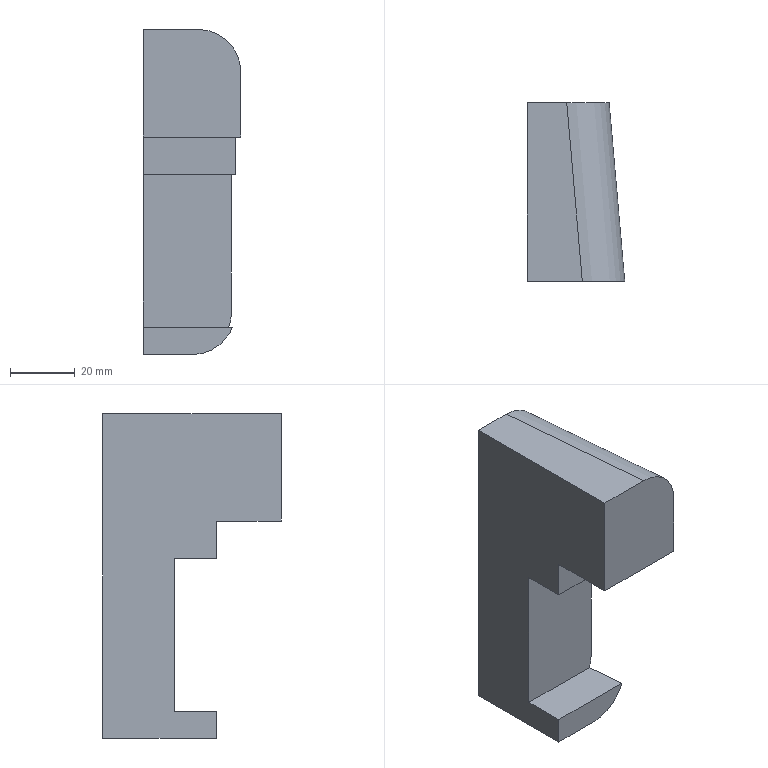Part | STEP file | 1 solid | 14 faces | box 30 x 55 x 100 mm | volume 92612 mm3 | plane 12 | cylinder 2 | commonest cylinder face diameters 26 x2
STEP:
#1=CARTESIAN_POINT('',(0.,0.,0.));
#2=DIRECTION('',(0.,0.,1.));
#3=DIRECTION('',(1.,0.,0.));
#4=AXIS2_PLACEMENT_3D('',#1,#2,#3);
#5=CARTESIAN_POINT('',(37.138,70.5,195.451));
#6=VERTEX_POINT('',#5);
#7=CARTESIAN_POINT('',(37.138,90.5,195.451));
#8=VERTEX_POINT('',#7);
#9=CARTESIAN_POINT('',(37.138,90.366,195.451));
#10=DIRECTION('',(0.,1.,0.));
#11=VECTOR('',#10,1.);
#12=LINE('',#9,#11);
#13=CARTESIAN_POINT('',(37.138,-9.5,128.53));
#14=DIRECTION('',(1.,0.,0.));
#15=DIRECTION('',(0.,0.,-1.));
#16=AXIS2_PLACEMENT_3D('',#13,#14,#15);
#17=PLANE('',#16);
#18=CARTESIAN_POINT('',(-66.922,99.866));
#19=DIRECTION('',(0.,1.));
#20=VECTOR('',#19,1.);
#21=LINE('',#18,#20);
#22=(GEOMETRIC_REPRESENTATION_CONTEXT(2)PARAMETRIC_REPRESENTATION_CONTEXT()REPRESENTATION_CONTEXT('',''));
#23=DEFINITIONAL_REPRESENTATION('',(#21),#22);
#24=PCURVE('',#17,#23);
#25=CARTESIAN_POINT('',(47.086,69.939,195.451));
#26=DIRECTION('',(0.,0.,-1.));
#27=DIRECTION('',(-1.,0.,0.));
#28=AXIS2_PLACEMENT_3D('',#25,#26,#27);
#29=PLANE('',#28);
#30=CARTESIAN_POINT('',(9.948,20.427));
#31=DIRECTION('',(0.,1.));
#32=VECTOR('',#31,1.);
#33=LINE('',#30,#32);
#34=(GEOMETRIC_REPRESENTATION_CONTEXT(2)PARAMETRIC_REPRESENTATION_CONTEXT()REPRESENTATION_CONTEXT('',''));
#35=DEFINITIONAL_REPRESENTATION('',(#33),#34);
#36=PCURVE('',#29,#35);
#37=SURFACE_CURVE('',#12,(#24,#36),.PCURVE_S1.);
#38=EDGE_CURVE('',#6,#8,#37,.T.);
#39=ORIENTED_EDGE('',*,*,#38,.F.);
#40=CARTESIAN_POINT('',(37.138,70.5,228.53));
#41=VERTEX_POINT('',#40);
#42=CARTESIAN_POINT('',(37.138,70.5,128.53));
#43=DIRECTION('',(0.,0.,1.));
#44=VECTOR('',#43,1.);
#45=LINE('',#42,#44);
#46=CARTESIAN_POINT('',(0.,80.));
#47=DIRECTION('',(-1.,0.));
#48=VECTOR('',#47,1.);
#49=LINE('',#46,#48);
#50=(GEOMETRIC_REPRESENTATION_CONTEXT(2)PARAMETRIC_REPRESENTATION_CONTEXT()REPRESENTATION_CONTEXT('',''));
#51=DEFINITIONAL_REPRESENTATION('',(#49),#50);
#52=PCURVE('',#17,#51);
#53=CARTESIAN_POINT('',(-72.862,70.5,-363.47));
#54=DIRECTION('',(0.,1.,0.));
#55=DIRECTION('',(0.,0.,-1.));
#56=AXIS2_PLACEMENT_3D('',#53,#54,#55);
#57=PLANE('',#56);
#58=CARTESIAN_POINT('',(-492.,-110.));
#59=DIRECTION('',(-1.,0.));
#60=VECTOR('',#59,1.);
#61=LINE('',#58,#60);
#62=(GEOMETRIC_REPRESENTATION_CONTEXT(2)PARAMETRIC_REPRESENTATION_CONTEXT()REPRESENTATION_CONTEXT('',''));
#63=DEFINITIONAL_REPRESENTATION('',(#61),#62);
#64=PCURVE('',#57,#63);
#65=SURFACE_CURVE('',#45,(#52,#64),.PCURVE_S1.);
#66=EDGE_CURVE('',#6,#41,#65,.T.);
#67=ORIENTED_EDGE('',*,*,#66,.T.);
#68=CARTESIAN_POINT('',(37.138,125.5,228.53));
#69=VERTEX_POINT('',#68);
#70=CARTESIAN_POINT('',(37.138,-9.5,228.53));
#71=DIRECTION('',(0.,1.,0.));
#72=VECTOR('',#71,1.);
#73=LINE('',#70,#72);
#74=CARTESIAN_POINT('',(-100.,0.));
#75=DIRECTION('',(0.,1.));
#76=VECTOR('',#75,1.);
#77=LINE('',#74,#76);
#78=(GEOMETRIC_REPRESENTATION_CONTEXT(2)PARAMETRIC_REPRESENTATION_CONTEXT()REPRESENTATION_CONTEXT('',''));
#79=DEFINITIONAL_REPRESENTATION('',(#77),#78);
#80=PCURVE('',#17,#79);
#81=CARTESIAN_POINT('',(37.138,-9.5,228.53));
#82=DIRECTION('',(0.,0.,-1.));
#83=DIRECTION('',(-1.,0.,0.));
#84=AXIS2_PLACEMENT_3D('',#81,#82,#83);
#85=PLANE('',#84);
#86=CARTESIAN_POINT('',(0.,0.));
#87=DIRECTION('',(0.,1.));
#88=VECTOR('',#87,1.);
#89=LINE('',#86,#88);
#90=(GEOMETRIC_REPRESENTATION_CONTEXT(2)PARAMETRIC_REPRESENTATION_CONTEXT()REPRESENTATION_CONTEXT('',''));
#91=DEFINITIONAL_REPRESENTATION('',(#89),#90);
#92=PCURVE('',#85,#91);
#93=SURFACE_CURVE('',#73,(#80,#92),.PCURVE_S1.);
#94=EDGE_CURVE('',#41,#69,#93,.T.);
#95=ORIENTED_EDGE('',*,*,#94,.T.);
#96=CARTESIAN_POINT('',(37.138,125.5,128.53));
#97=VERTEX_POINT('',#96);
#98=CARTESIAN_POINT('',(37.138,125.5,128.53));
#99=DIRECTION('',(0.,0.,-1.));
#100=VECTOR('',#99,1.);
#101=LINE('',#98,#100);
#102=CARTESIAN_POINT('',(0.,135.));
#103=DIRECTION('',(1.,0.));
#104=VECTOR('',#103,1.);
#105=LINE('',#102,#104);
#106=(GEOMETRIC_REPRESENTATION_CONTEXT(2)PARAMETRIC_REPRESENTATION_CONTEXT()REPRESENTATION_CONTEXT('',''));
#107=DEFINITIONAL_REPRESENTATION('',(#105),#106);
#108=PCURVE('',#17,#107);
#109=CARTESIAN_POINT('',(-72.362,125.5,-51.47));
#110=DIRECTION('',(0.,-1.,0.));
#111=DIRECTION('',(0.,0.,-1.));
#112=AXIS2_PLACEMENT_3D('',#109,#110,#111);
#113=PLANE('',#112);
#114=CARTESIAN_POINT('',(-180.,109.5));
#115=DIRECTION('',(1.,0.));
#116=VECTOR('',#115,1.);
#117=LINE('',#114,#116);
#118=(GEOMETRIC_REPRESENTATION_CONTEXT(2)PARAMETRIC_REPRESENTATION_CONTEXT()REPRESENTATION_CONTEXT('',''));
#119=DEFINITIONAL_REPRESENTATION('',(#117),#118);
#120=PCURVE('',#113,#119);
#121=SURFACE_CURVE('',#101,(#108,#120),.PCURVE_S1.);
#122=EDGE_CURVE('',#69,#97,#121,.T.);
#123=ORIENTED_EDGE('',*,*,#122,.T.);
#124=CARTESIAN_POINT('',(37.138,90.5,128.53));
#125=VERTEX_POINT('',#124);
#126=CARTESIAN_POINT('',(37.138,-9.5,128.53));
#127=DIRECTION('',(0.,1.,0.));
#128=VECTOR('',#127,1.);
#129=LINE('',#126,#128);
#130=CARTESIAN_POINT('',(0.,0.));
#131=DIRECTION('',(0.,1.));
#132=VECTOR('',#131,1.);
#133=LINE('',#130,#132);
#134=(GEOMETRIC_REPRESENTATION_CONTEXT(2)PARAMETRIC_REPRESENTATION_CONTEXT()REPRESENTATION_CONTEXT('',''));
#135=DEFINITIONAL_REPRESENTATION('',(#133),#134);
#136=PCURVE('',#17,#135);
#137=CARTESIAN_POINT('',(57.138,-9.5,128.53));
#138=DIRECTION('',(0.,0.,1.));
#139=DIRECTION('',(1.,0.,0.));
#140=AXIS2_PLACEMENT_3D('',#137,#138,#139);
#141=PLANE('',#140);
#142=CARTESIAN_POINT('',(-20.,0.));
#143=DIRECTION('',(0.,1.));
#144=VECTOR('',#143,1.);
#145=LINE('',#142,#144);
#146=(GEOMETRIC_REPRESENTATION_CONTEXT(2)PARAMETRIC_REPRESENTATION_CONTEXT()REPRESENTATION_CONTEXT('',''));
#147=DEFINITIONAL_REPRESENTATION('',(#145),#146);
#148=PCURVE('',#141,#147);
#149=SURFACE_CURVE('',#129,(#136,#148),.PCURVE_S1.);
#150=EDGE_CURVE('',#125,#97,#149,.T.);
#151=ORIENTED_EDGE('',*,*,#150,.F.);
#152=CARTESIAN_POINT('',(37.138,90.5,136.951));
#153=VERTEX_POINT('',#152);
#154=CARTESIAN_POINT('',(37.138,90.5,128.53));
#155=DIRECTION('',(0.,0.,1.));
#156=VECTOR('',#155,1.);
#157=LINE('',#154,#156);
#158=CARTESIAN_POINT('',(0.,100.));
#159=DIRECTION('',(-1.,0.));
#160=VECTOR('',#159,1.);
#161=LINE('',#158,#160);
#162=(GEOMETRIC_REPRESENTATION_CONTEXT(2)PARAMETRIC_REPRESENTATION_CONTEXT()REPRESENTATION_CONTEXT('',''));
#163=DEFINITIONAL_REPRESENTATION('',(#161),#162);
#164=PCURVE('',#17,#163);
#165=CARTESIAN_POINT('',(47.086,90.5,125.451));
#166=DIRECTION('',(0.,1.,0.));
#167=DIRECTION('',(0.,0.,1.));
#168=AXIS2_PLACEMENT_3D('',#165,#166,#167);
#169=PLANE('',#168);
#170=CARTESIAN_POINT('',(3.078,-9.948));
#171=DIRECTION('',(1.,0.));
#172=VECTOR('',#171,1.);
#173=LINE('',#170,#172);
#174=(GEOMETRIC_REPRESENTATION_CONTEXT(2)PARAMETRIC_REPRESENTATION_CONTEXT()REPRESENTATION_CONTEXT('',''));
#175=DEFINITIONAL_REPRESENTATION('',(#173),#174);
#176=PCURVE('',#169,#175);
#177=SURFACE_CURVE('',#157,(#164,#176),.PCURVE_S1.);
#178=EDGE_CURVE('',#125,#153,#177,.T.);
#179=ORIENTED_EDGE('',*,*,#178,.T.);
#180=CARTESIAN_POINT('',(37.138,103.5,136.951));
#181=VERTEX_POINT('',#180);
#182=CARTESIAN_POINT('',(37.138,69.939,136.951));
#183=DIRECTION('',(0.,1.,0.));
#184=VECTOR('',#183,1.);
#185=LINE('',#182,#184);
#186=CARTESIAN_POINT('',(-8.422,79.439));
#187=DIRECTION('',(0.,1.));
#188=VECTOR('',#187,1.);
#189=LINE('',#186,#188);
#190=(GEOMETRIC_REPRESENTATION_CONTEXT(2)PARAMETRIC_REPRESENTATION_CONTEXT()REPRESENTATION_CONTEXT('',''));
#191=DEFINITIONAL_REPRESENTATION('',(#189),#190);
#192=PCURVE('',#17,#191);
#193=CARTESIAN_POINT('',(47.085,69.939,136.951));
#194=DIRECTION('',(0.,0.,1.));
#195=DIRECTION('',(-1.,0.,0.));
#196=AXIS2_PLACEMENT_3D('',#193,#194,#195);
#197=PLANE('',#196);
#198=CARTESIAN_POINT('',(9.948,0.));
#199=DIRECTION('',(0.,-1.));
#200=VECTOR('',#199,1.);
#201=LINE('',#198,#200);
#202=(GEOMETRIC_REPRESENTATION_CONTEXT(2)PARAMETRIC_REPRESENTATION_CONTEXT()REPRESENTATION_CONTEXT('',''));
#203=DEFINITIONAL_REPRESENTATION('',(#201),#202);
#204=PCURVE('',#197,#203);
#205=SURFACE_CURVE('',#185,(#192,#204),.PCURVE_S1.);
#206=EDGE_CURVE('',#153,#181,#205,.T.);
#207=ORIENTED_EDGE('',*,*,#206,.T.);
#208=CARTESIAN_POINT('',(37.138,103.5,183.951));
#209=VERTEX_POINT('',#208);
#210=CARTESIAN_POINT('',(37.138,103.5,128.53));
#211=DIRECTION('',(0.,0.,-1.));
#212=VECTOR('',#211,1.);
#213=LINE('',#210,#212);
#214=CARTESIAN_POINT('',(0.,113.));
#215=DIRECTION('',(1.,0.));
#216=VECTOR('',#215,1.);
#217=LINE('',#214,#216);
#218=(GEOMETRIC_REPRESENTATION_CONTEXT(2)PARAMETRIC_REPRESENTATION_CONTEXT()REPRESENTATION_CONTEXT('',''));
#219=DEFINITIONAL_REPRESENTATION('',(#217),#218);
#220=PCURVE('',#17,#219);
#221=CARTESIAN_POINT('',(87.138,103.5,108.53));
#222=DIRECTION('',(0.,-1.,0.));
#223=DIRECTION('',(0.,0.,-1.));
#224=AXIS2_PLACEMENT_3D('',#221,#222,#223);
#225=PLANE('',#224);
#226=CARTESIAN_POINT('',(-20.,-50.));
#227=DIRECTION('',(1.,0.));
#228=VECTOR('',#227,1.);
#229=LINE('',#226,#228);
#230=(GEOMETRIC_REPRESENTATION_CONTEXT(2)PARAMETRIC_REPRESENTATION_CONTEXT()REPRESENTATION_CONTEXT('',''));
#231=DEFINITIONAL_REPRESENTATION('',(#229),#230);
#232=PCURVE('',#225,#231);
#233=SURFACE_CURVE('',#213,(#220,#232),.PCURVE_S1.);
#234=EDGE_CURVE('',#209,#181,#233,.T.);
#235=ORIENTED_EDGE('',*,*,#234,.F.);
#236=CARTESIAN_POINT('',(37.138,90.5,183.951));
#237=VERTEX_POINT('',#236);
#238=CARTESIAN_POINT('',(37.138,69.939,183.951));
#239=DIRECTION('',(0.,1.,0.));
#240=VECTOR('',#239,1.);
#241=LINE('',#238,#240);
#242=CARTESIAN_POINT('',(-55.422,79.439));
#243=DIRECTION('',(0.,1.));
#244=VECTOR('',#243,1.);
#245=LINE('',#242,#244);
#246=(GEOMETRIC_REPRESENTATION_CONTEXT(2)PARAMETRIC_REPRESENTATION_CONTEXT()REPRESENTATION_CONTEXT('',''));
#247=DEFINITIONAL_REPRESENTATION('',(#245),#246);
#248=PCURVE('',#17,#247);
#249=CARTESIAN_POINT('',(47.085,69.939,183.951));
#250=DIRECTION('',(0.,0.,1.));
#251=DIRECTION('',(-1.,0.,0.));
#252=AXIS2_PLACEMENT_3D('',#249,#250,#251);
#253=PLANE('',#252);
#254=CARTESIAN_POINT('',(9.948,0.));
#255=DIRECTION('',(0.,-1.));
#256=VECTOR('',#255,1.);
#257=LINE('',#254,#256);
#258=(GEOMETRIC_REPRESENTATION_CONTEXT(2)PARAMETRIC_REPRESENTATION_CONTEXT()REPRESENTATION_CONTEXT('',''));
#259=DEFINITIONAL_REPRESENTATION('',(#257),#258);
#260=PCURVE('',#253,#259);
#261=SURFACE_CURVE('',#241,(#248,#260),.PCURVE_S1.);
#262=EDGE_CURVE('',#237,#209,#261,.T.);
#263=ORIENTED_EDGE('',*,*,#262,.F.);
#264=CARTESIAN_POINT('',(37.138,90.5,195.451));
#265=DIRECTION('',(0.,0.,-1.));
#266=VECTOR('',#265,1.);
#267=LINE('',#264,#266);
#268=CARTESIAN_POINT('',(-66.922,100.));
#269=DIRECTION('',(1.,0.));
#270=VECTOR('',#269,1.);
#271=LINE('',#268,#270);
#272=(GEOMETRIC_REPRESENTATION_CONTEXT(2)PARAMETRIC_REPRESENTATION_CONTEXT()REPRESENTATION_CONTEXT('',''));
#273=DEFINITIONAL_REPRESENTATION('',(#271),#272);
#274=PCURVE('',#17,#273);
#275=CARTESIAN_POINT('',(47.086,90.5,195.451));
#276=DIRECTION('',(0.,1.,0.));
#277=DIRECTION('',(0.,0.,-1.));
#278=AXIS2_PLACEMENT_3D('',#275,#276,#277);
#279=PLANE('',#278);
#280=CARTESIAN_POINT('',(0.,9.948));
#281=DIRECTION('',(1.,0.));
#282=VECTOR('',#281,1.);
#283=LINE('',#280,#282);
#284=(GEOMETRIC_REPRESENTATION_CONTEXT(2)PARAMETRIC_REPRESENTATION_CONTEXT()REPRESENTATION_CONTEXT('',''));
#285=DEFINITIONAL_REPRESENTATION('',(#283),#284);
#286=PCURVE('',#279,#285);
#287=SURFACE_CURVE('',#267,(#274,#286),.PCURVE_S1.);
#288=EDGE_CURVE('',#8,#237,#287,.T.);
#289=ORIENTED_EDGE('',*,*,#288,.F.);
#290=EDGE_LOOP('',(#39,#67,#95,#123,#151,#179,#207,#235,#263,#289));
#291=FACE_BOUND('',#290,.T.);
#292=ADVANCED_FACE('',(#291),#17,.F.);
#293=CARTESIAN_POINT('',(52.338,90.5,128.53));
#294=VERTEX_POINT('',#293);
#295=CARTESIAN_POINT('',(64.552,90.5,136.951));
#296=VERTEX_POINT('',#295);
#297=CARTESIAN_POINT('',(52.338,90.5,128.53));
#298=CARTESIAN_POINT('',(57.955,90.5,128.53));
#299=CARTESIAN_POINT('',(62.574,90.5,131.714));
#300=CARTESIAN_POINT('',(64.552,90.5,136.951));
#301=(BOUNDED_CURVE()B_SPLINE_CURVE(3,(#297,#298,#299,#300),.UNSPECIFIED.,.F.,.F.)B_SPLINE_CURVE_WITH_KNOTS((4,4),(1.571,2.782),.PIECEWISE_BEZIER_KNOTS.)CURVE()GEOMETRIC_REPRESENTATION_ITEM()RATIONAL_B_SPLINE_CURVE((1.,0.8815,0.8815,1.))REPRESENTATION_ITEM(''));
#302=CARTESIAN_POINT('',(61.057,-9.157,141.53));
#303=DIRECTION('',(-0.08716,0.9962,0.));
#304=DIRECTION('',(0.9962,0.08716,0.));
#305=AXIS2_PLACEMENT_3D('',#302,#303,#304);
#306=CYLINDRICAL_SURFACE('',#305,13.);
#307=CARTESIAN_POINT('',(1.571,100.038));
#308=CARTESIAN_POINT('',(1.554,100.018));
#309=CARTESIAN_POINT('',(1.519,99.979));
#310=CARTESIAN_POINT('',(1.466,99.919));
#311=CARTESIAN_POINT('',(1.412,99.858));
#312=CARTESIAN_POINT('',(1.358,99.797));
#313=CARTESIAN_POINT('',(1.303,99.737));
#314=CARTESIAN_POINT('',(1.247,99.676));
#315=CARTESIAN_POINT('',(1.192,99.617));
#316=CARTESIAN_POINT('',(1.135,99.558));
#317=CARTESIAN_POINT('',(1.079,99.5));
#318=CARTESIAN_POINT('',(1.022,99.444));
#319=CARTESIAN_POINT('',(0.9653,99.39));
#320=CARTESIAN_POINT('',(0.9086,99.338));
#321=CARTESIAN_POINT('',(0.8519,99.288));
#322=CARTESIAN_POINT('',(0.7954,99.241));
#323=CARTESIAN_POINT('',(0.7391,99.197));
#324=CARTESIAN_POINT('',(0.6832,99.155));
#325=CARTESIAN_POINT('',(0.6278,99.117));
#326=CARTESIAN_POINT('',(0.5729,99.082));
#327=CARTESIAN_POINT('',(0.5185,99.049));
#328=CARTESIAN_POINT('',(0.4649,99.021));
#329=CARTESIAN_POINT('',(0.4119,98.995));
#330=CARTESIAN_POINT('',(0.3771,98.98));
#331=CARTESIAN_POINT('',(0.3599,98.973));
#332=B_SPLINE_CURVE_WITH_KNOTS('',3,(#307,#308,#309,#310,#311,#312,#313,#314,#315,#316,#317,#318,#319,#320,#321,#322,#323,#324,#325,#326,#327,#328,#329,#330,#331),.UNSPECIFIED.,.F.,.F.,(4,1,1,1,1,1,1,1,1,1,1,1,1,1,1,1,1,1,1,1,1,1,4),(1.571,1.626,1.681,1.736,1.791,1.846,1.901,1.956,2.011,2.066,2.121,2.176,2.231,2.286,2.341,2.396,2.451,2.506,2.562,2.617,2.672,2.727,2.782),.QUASI_UNIFORM_KNOTS.);
#333=(GEOMETRIC_REPRESENTATION_CONTEXT(2)PARAMETRIC_REPRESENTATION_CONTEXT()REPRESENTATION_CONTEXT('',''));
#334=DEFINITIONAL_REPRESENTATION('',(#332),#333);
#335=PCURVE('',#306,#334);
#336=CARTESIAN_POINT('',(3.078,5.253));
#337=CARTESIAN_POINT('',(3.078,10.87));
#338=CARTESIAN_POINT('',(6.263,15.488));
#339=CARTESIAN_POINT('',(11.5,17.466));
#340=(BOUNDED_CURVE()B_SPLINE_CURVE(3,(#336,#337,#338,#339),.UNSPECIFIED.,.F.,.F.)B_SPLINE_CURVE_WITH_KNOTS((4,4),(1.571,2.782),.PIECEWISE_BEZIER_KNOTS.)CURVE()GEOMETRIC_REPRESENTATION_ITEM()RATIONAL_B_SPLINE_CURVE((1.,0.8815,0.8815,1.))REPRESENTATION_ITEM(''));
#341=(GEOMETRIC_REPRESENTATION_CONTEXT(2)PARAMETRIC_REPRESENTATION_CONTEXT()REPRESENTATION_CONTEXT('',''));
#342=DEFINITIONAL_REPRESENTATION('',(#340),#341);
#343=PCURVE('',#169,#342);
#344=SURFACE_CURVE('',#301,(#335,#343),.PCURVE_S1.);
#345=EDGE_CURVE('',#294,#296,#344,.T.);
#346=ORIENTED_EDGE('',*,*,#345,.F.);
#347=CARTESIAN_POINT('',(49.276,125.5,128.53));
#348=VERTEX_POINT('',#347);
#349=CARTESIAN_POINT('',(61.057,-9.157,128.53));
#350=DIRECTION('',(-0.08716,0.9962,0.));
#351=VECTOR('',#350,1.);
#352=LINE('',#349,#351);
#353=CARTESIAN_POINT('',(1.571,0.));
#354=DIRECTION('',(0.,1.));
#355=VECTOR('',#354,1.);
#356=LINE('',#353,#355);
#357=(GEOMETRIC_REPRESENTATION_CONTEXT(2)PARAMETRIC_REPRESENTATION_CONTEXT()REPRESENTATION_CONTEXT('',''));
#358=DEFINITIONAL_REPRESENTATION('',(#356),#357);
#359=PCURVE('',#306,#358);
#360=CARTESIAN_POINT('',(3.919,0.3429));
#361=DIRECTION('',(-0.08716,0.9962));
#362=VECTOR('',#361,1.);
#363=LINE('',#360,#362);
#364=(GEOMETRIC_REPRESENTATION_CONTEXT(2)PARAMETRIC_REPRESENTATION_CONTEXT()REPRESENTATION_CONTEXT('',''));
#365=DEFINITIONAL_REPRESENTATION('',(#363),#364);
#366=PCURVE('',#141,#365);
#367=SURFACE_CURVE('',#352,(#359,#366),.PCURVE_S1.);
#368=EDGE_CURVE('',#294,#348,#367,.T.);
#369=ORIENTED_EDGE('',*,*,#368,.T.);
#370=CARTESIAN_POINT('',(62.326,125.5,141.53));
#371=VERTEX_POINT('',#370);
#372=CARTESIAN_POINT('',(62.326,125.5,141.53));
#373=CARTESIAN_POINT('',(62.326,125.5,133.914));
#374=CARTESIAN_POINT('',(56.92,125.5,128.53));
#375=CARTESIAN_POINT('',(49.276,125.5,128.53));
#376=(BOUNDED_CURVE()B_SPLINE_CURVE(3,(#372,#373,#374,#375),.UNSPECIFIED.,.F.,.F.)B_SPLINE_CURVE_WITH_KNOTS((4,4),(3.142,4.712),.PIECEWISE_BEZIER_KNOTS.)CURVE()GEOMETRIC_REPRESENTATION_ITEM()RATIONAL_B_SPLINE_CURVE((1.,0.8047,0.8047,1.))REPRESENTATION_ITEM(''));
#377=CARTESIAN_POINT('',(0.,134.034));
#378=CARTESIAN_POINT('',(0.02143,134.034));
#379=CARTESIAN_POINT('',(0.06485,134.036));
#380=CARTESIAN_POINT('',(0.1316,134.043));
#381=CARTESIAN_POINT('',(0.2,134.056));
#382=CARTESIAN_POINT('',(0.2697,134.074));
#383=CARTESIAN_POINT('',(0.3408,134.099));
#384=CARTESIAN_POINT('',(0.413,134.129));
#385=CARTESIAN_POINT('',(0.4863,134.165));
#386=CARTESIAN_POINT('',(0.5603,134.207));
#387=CARTESIAN_POINT('',(0.635,134.255));
#388=CARTESIAN_POINT('',(0.7101,134.308));
#389=CARTESIAN_POINT('',(0.7854,134.366));
#390=CARTESIAN_POINT('',(0.8607,134.429));
#391=CARTESIAN_POINT('',(0.9358,134.496));
#392=CARTESIAN_POINT('',(1.01,134.566));
#393=CARTESIAN_POINT('',(1.085,134.639));
#394=CARTESIAN_POINT('',(1.158,134.715));
#395=CARTESIAN_POINT('',(1.23,134.791));
#396=CARTESIAN_POINT('',(1.301,134.868));
#397=CARTESIAN_POINT('',(1.371,134.945));
#398=CARTESIAN_POINT('',(1.439,135.022));
#399=CARTESIAN_POINT('',(1.506,135.098));
#400=CARTESIAN_POINT('',(1.549,135.147));
#401=CARTESIAN_POINT('',(1.571,135.171));
#402=B_SPLINE_CURVE_WITH_KNOTS('',3,(#377,#378,#379,#380,#381,#382,#383,#384,#385,#386,#387,#388,#389,#390,#391,#392,#393,#394,#395,#396,#397,#398,#399,#400,#401),.UNSPECIFIED.,.F.,.F.,(4,1,1,1,1,1,1,1,1,1,1,1,1,1,1,1,1,1,1,1,1,1,4),(3.142,3.213,3.284,3.356,3.427,3.499,3.57,3.641,3.713,3.784,3.856,3.927,3.998,4.07,4.141,4.213,4.284,4.355,4.427,4.498,4.57,4.641,4.712),.QUASI_UNIFORM_KNOTS.);
#403=(GEOMETRIC_REPRESENTATION_CONTEXT(2)PARAMETRIC_REPRESENTATION_CONTEXT()REPRESENTATION_CONTEXT('',''));
#404=DEFINITIONAL_REPRESENTATION('',(#402),#403);
#405=PCURVE('',#306,#404);
#406=CARTESIAN_POINT('',(-193.,134.688));
#407=CARTESIAN_POINT('',(-185.385,134.688));
#408=CARTESIAN_POINT('',(-180.,129.283));
#409=CARTESIAN_POINT('',(-180.,121.638));
#410=(BOUNDED_CURVE()B_SPLINE_CURVE(3,(#406,#407,#408,#409),.UNSPECIFIED.,.F.,.F.)B_SPLINE_CURVE_WITH_KNOTS((4,4),(3.142,4.712),.PIECEWISE_BEZIER_KNOTS.)CURVE()GEOMETRIC_REPRESENTATION_ITEM()RATIONAL_B_SPLINE_CURVE((1.,0.8047,0.8047,1.))REPRESENTATION_ITEM(''));
#411=(GEOMETRIC_REPRESENTATION_CONTEXT(2)PARAMETRIC_REPRESENTATION_CONTEXT()REPRESENTATION_CONTEXT('',''));
#412=DEFINITIONAL_REPRESENTATION('',(#410),#411);
#413=PCURVE('',#113,#412);
#414=SURFACE_CURVE('',#376,(#405,#413),.PCURVE_S1.);
#415=EDGE_CURVE('',#371,#348,#414,.T.);
#416=ORIENTED_EDGE('',*,*,#415,.F.);
#417=CARTESIAN_POINT('',(64.25,103.5,141.53));
#418=VERTEX_POINT('',#417);
#419=CARTESIAN_POINT('',(67.138,70.5,141.53));
#420=DIRECTION('',(0.08716,-0.9962,0.));
#421=VECTOR('',#420,1.);
#422=LINE('',#419,#421);
#423=CARTESIAN_POINT('',(0.,78.824));
#424=DIRECTION('',(0.,-1.));
#425=VECTOR('',#424,1.);
#426=LINE('',#423,#425);
#427=(GEOMETRIC_REPRESENTATION_CONTEXT(2)PARAMETRIC_REPRESENTATION_CONTEXT()REPRESENTATION_CONTEXT('',''));
#428=DEFINITIONAL_REPRESENTATION('',(#426),#427);
#429=PCURVE('',#306,#428);
#430=CARTESIAN_POINT('',(67.138,70.5,178.53));
#431=DIRECTION('',(-0.9962,-0.08716,0.));
#432=DIRECTION('',(-0.08716,0.9962,0.));
#433=AXIS2_PLACEMENT_3D('',#430,#431,#432);
#434=PLANE('',#433);
#435=CARTESIAN_POINT('',(0.,37.));
#436=DIRECTION('',(-1.,0.));
#437=VECTOR('',#436,1.);
#438=LINE('',#435,#437);
#439=(GEOMETRIC_REPRESENTATION_CONTEXT(2)PARAMETRIC_REPRESENTATION_CONTEXT()REPRESENTATION_CONTEXT('',''));
#440=DEFINITIONAL_REPRESENTATION('',(#438),#439);
#441=PCURVE('',#434,#440);
#442=SURFACE_CURVE('',#422,(#429,#441),.PCURVE_S1.);
#443=EDGE_CURVE('',#371,#418,#442,.T.);
#444=ORIENTED_EDGE('',*,*,#443,.T.);
#445=CARTESIAN_POINT('',(63.414,103.5,136.951));
#446=VERTEX_POINT('',#445);
#447=CARTESIAN_POINT('',(64.25,103.5,141.53));
#448=CARTESIAN_POINT('',(64.25,103.5,139.962));
#449=CARTESIAN_POINT('',(63.969,103.5,138.419));
#450=CARTESIAN_POINT('',(63.414,103.5,136.951));
#451=(BOUNDED_CURVE()B_SPLINE_CURVE(3,(#447,#448,#449,#450),.UNSPECIFIED.,.F.,.F.)B_SPLINE_CURVE_WITH_KNOTS((4,4),(3.142,3.501),.PIECEWISE_BEZIER_KNOTS.)CURVE()GEOMETRIC_REPRESENTATION_ITEM()RATIONAL_B_SPLINE_CURVE((1.,0.9892,0.9892,1.))REPRESENTATION_ITEM(''));
#452=CARTESIAN_POINT('',(0.,111.95));
#453=CARTESIAN_POINT('',(0.005424,111.95));
#454=CARTESIAN_POINT('',(0.01628,111.95));
#455=CARTESIAN_POINT('',(0.03258,111.951));
#456=CARTESIAN_POINT('',(0.04891,111.951));
#457=CARTESIAN_POINT('',(0.06525,111.952));
#458=CARTESIAN_POINT('',(0.08161,111.954));
#459=CARTESIAN_POINT('',(0.09798,111.955));
#460=CARTESIAN_POINT('',(0.1144,111.957));
#461=CARTESIAN_POINT('',(0.1307,111.96));
#462=CARTESIAN_POINT('',(0.1471,111.962));
#463=CARTESIAN_POINT('',(0.1635,111.965));
#464=CARTESIAN_POINT('',(0.1799,111.968));
#465=CARTESIAN_POINT('',(0.1964,111.972));
#466=CARTESIAN_POINT('',(0.2128,111.976));
#467=CARTESIAN_POINT('',(0.2291,111.98));
#468=CARTESIAN_POINT('',(0.2455,111.984));
#469=CARTESIAN_POINT('',(0.2619,111.989));
#470=CARTESIAN_POINT('',(0.2783,111.994));
#471=CARTESIAN_POINT('',(0.2946,111.999));
#472=CARTESIAN_POINT('',(0.311,112.005));
#473=CARTESIAN_POINT('',(0.3273,112.01));
#474=CARTESIAN_POINT('',(0.3436,112.017));
#475=CARTESIAN_POINT('',(0.3545,112.021));
#476=CARTESIAN_POINT('',(0.3599,112.023));
#477=B_SPLINE_CURVE_WITH_KNOTS('',3,(#452,#453,#454,#455,#456,#457,#458,#459,#460,#461,#462,#463,#464,#465,#466,#467,#468,#469,#470,#471,#472,#473,#474,#475,#476),.UNSPECIFIED.,.F.,.F.,(4,1,1,1,1,1,1,1,1,1,1,1,1,1,1,1,1,1,1,1,1,1,4),(3.142,3.158,3.174,3.191,3.207,3.223,3.24,3.256,3.272,3.289,3.305,3.322,3.338,3.354,3.371,3.387,3.403,3.42,3.436,3.452,3.469,3.485,3.501),.QUASI_UNIFORM_KNOTS.);
#478=(GEOMETRIC_REPRESENTATION_CONTEXT(2)PARAMETRIC_REPRESENTATION_CONTEXT()REPRESENTATION_CONTEXT('',''));
#479=DEFINITIONAL_REPRESENTATION('',(#477),#478);
#480=PCURVE('',#306,#479);
#481=CARTESIAN_POINT('',(-33.,-22.887));
#482=CARTESIAN_POINT('',(-31.432,-22.887));
#483=CARTESIAN_POINT('',(-29.889,-23.169));
#484=CARTESIAN_POINT('',(-28.422,-23.723));
#485=(BOUNDED_CURVE()B_SPLINE_CURVE(3,(#481,#482,#483,#484),.UNSPECIFIED.,.F.,.F.)B_SPLINE_CURVE_WITH_KNOTS((4,4),(3.142,3.501),.PIECEWISE_BEZIER_KNOTS.)CURVE()GEOMETRIC_REPRESENTATION_ITEM()RATIONAL_B_SPLINE_CURVE((1.,0.9892,0.9892,1.))REPRESENTATION_ITEM(''));
#486=(GEOMETRIC_REPRESENTATION_CONTEXT(2)PARAMETRIC_REPRESENTATION_CONTEXT()REPRESENTATION_CONTEXT('',''));
#487=DEFINITIONAL_REPRESENTATION('',(#485),#486);
#488=PCURVE('',#225,#487);
#489=SURFACE_CURVE('',#451,(#480,#488),.PCURVE_S1.);
#490=EDGE_CURVE('',#418,#446,#489,.T.);
#491=ORIENTED_EDGE('',*,*,#490,.T.);
#492=CARTESIAN_POINT('',(73.178,-8.097,136.951));
#493=DIRECTION('',(0.08716,-0.9962,0.));
#494=VECTOR('',#493,1.);
#495=LINE('',#492,#494);
#496=CARTESIAN_POINT('',(0.3599,0.));
#497=DIRECTION('',(0.,-1.));
#498=VECTOR('',#497,1.);
#499=LINE('',#496,#498);
#500=(GEOMETRIC_REPRESENTATION_CONTEXT(2)PARAMETRIC_REPRESENTATION_CONTEXT()REPRESENTATION_CONTEXT('',''));
#501=DEFINITIONAL_REPRESENTATION('',(#499),#500);
#502=PCURVE('',#306,#501);
#503=CARTESIAN_POINT('',(-26.092,78.036));
#504=DIRECTION('',(-0.08716,0.9962));
#505=VECTOR('',#504,1.);
#506=LINE('',#503,#505);
#507=(GEOMETRIC_REPRESENTATION_CONTEXT(2)PARAMETRIC_REPRESENTATION_CONTEXT()REPRESENTATION_CONTEXT('',''));
#508=DEFINITIONAL_REPRESENTATION('',(#506),#507);
#509=PCURVE('',#197,#508);
#510=SURFACE_CURVE('',#495,(#502,#509),.PCURVE_S1.);
#511=EDGE_CURVE('',#446,#296,#510,.T.);
#512=ORIENTED_EDGE('',*,*,#511,.T.);
#513=EDGE_LOOP('',(#346,#369,#416,#444,#491,#512));
#514=FACE_BOUND('',#513,.T.);
#515=ADVANCED_FACE('',(#514),#306,.T.);
#516=CARTESIAN_POINT('',(67.138,70.5,195.451));
#517=VERTEX_POINT('',#516);
#518=CARTESIAN_POINT('',(-72.863,70.5,195.451));
#519=DIRECTION('',(-1.,0.,0.));
#520=VECTOR('',#519,1.);
#521=LINE('',#518,#520);
#522=CARTESIAN_POINT('',(-558.922,0.));
#523=DIRECTION('',(0.,1.));
#524=VECTOR('',#523,1.);
#525=LINE('',#522,#524);
#526=(GEOMETRIC_REPRESENTATION_CONTEXT(2)PARAMETRIC_REPRESENTATION_CONTEXT()REPRESENTATION_CONTEXT('',''));
#527=DEFINITIONAL_REPRESENTATION('',(#525),#526);
#528=PCURVE('',#57,#527);
#529=CARTESIAN_POINT('',(119.948,0.561));
#530=DIRECTION('',(1.,0.));
#531=VECTOR('',#530,1.);
#532=LINE('',#529,#531);
#533=(GEOMETRIC_REPRESENTATION_CONTEXT(2)PARAMETRIC_REPRESENTATION_CONTEXT()REPRESENTATION_CONTEXT('',''));
#534=DEFINITIONAL_REPRESENTATION('',(#532),#533);
#535=PCURVE('',#29,#534);
#536=SURFACE_CURVE('',#521,(#528,#535),.PCURVE_S1.);
#537=EDGE_CURVE('',#517,#6,#536,.T.);
#538=ORIENTED_EDGE('',*,*,#537,.F.);
#539=CARTESIAN_POINT('',(67.138,70.5,215.53));
#540=VERTEX_POINT('',#539);
#541=CARTESIAN_POINT('',(67.138,70.5,178.53));
#542=DIRECTION('',(0.,0.,-1.));
#543=VECTOR('',#542,1.);
#544=LINE('',#541,#543);
#545=CARTESIAN_POINT('',(-542.,-140.));
#546=DIRECTION('',(1.,0.));
#547=VECTOR('',#546,1.);
#548=LINE('',#545,#547);
#549=(GEOMETRIC_REPRESENTATION_CONTEXT(2)PARAMETRIC_REPRESENTATION_CONTEXT()REPRESENTATION_CONTEXT('',''));
#550=DEFINITIONAL_REPRESENTATION('',(#548),#549);
#551=PCURVE('',#57,#550);
#552=CARTESIAN_POINT('',(0.,0.));
#553=DIRECTION('',(0.,1.));
#554=VECTOR('',#553,1.);
#555=LINE('',#552,#554);
#556=(GEOMETRIC_REPRESENTATION_CONTEXT(2)PARAMETRIC_REPRESENTATION_CONTEXT()REPRESENTATION_CONTEXT('',''));
#557=DEFINITIONAL_REPRESENTATION('',(#555),#556);
#558=PCURVE('',#434,#557);
#559=SURFACE_CURVE('',#544,(#551,#558),.PCURVE_S1.);
#560=EDGE_CURVE('',#540,#517,#559,.T.);
#561=ORIENTED_EDGE('',*,*,#560,.F.);
#562=CARTESIAN_POINT('',(54.088,70.5,228.53));
#563=VERTEX_POINT('',#562);
#564=CARTESIAN_POINT('',(54.088,70.5,228.53));
#565=CARTESIAN_POINT('',(61.732,70.5,228.53));
#566=CARTESIAN_POINT('',(67.138,70.5,223.145));
#567=CARTESIAN_POINT('',(67.138,70.5,215.53));
#568=(BOUNDED_CURVE()B_SPLINE_CURVE(3,(#564,#565,#566,#567),.UNSPECIFIED.,.F.,.F.)B_SPLINE_CURVE_WITH_KNOTS((4,4),(1.571,3.142),.PIECEWISE_BEZIER_KNOTS.)CURVE()GEOMETRIC_REPRESENTATION_ITEM()RATIONAL_B_SPLINE_CURVE((1.,0.8047,0.8047,1.))REPRESENTATION_ITEM(''));
#569=CARTESIAN_POINT('',(-592.,-126.95));
#570=CARTESIAN_POINT('',(-592.,-134.595));
#571=CARTESIAN_POINT('',(-586.615,-140.));
#572=CARTESIAN_POINT('',(-579.,-140.));
#573=(BOUNDED_CURVE()B_SPLINE_CURVE(3,(#569,#570,#571,#572),.UNSPECIFIED.,.F.,.F.)B_SPLINE_CURVE_WITH_KNOTS((4,4),(1.571,3.142),.PIECEWISE_BEZIER_KNOTS.)CURVE()GEOMETRIC_REPRESENTATION_ITEM()RATIONAL_B_SPLINE_CURVE((1.,0.8047,0.8047,1.))REPRESENTATION_ITEM(''));
#574=(GEOMETRIC_REPRESENTATION_CONTEXT(2)PARAMETRIC_REPRESENTATION_CONTEXT()REPRESENTATION_CONTEXT('',''));
#575=DEFINITIONAL_REPRESENTATION('',(#573),#574);
#576=PCURVE('',#57,#575);
#577=CARTESIAN_POINT('',(54.187,69.367,215.53));
#578=DIRECTION('',(-0.08716,0.9962,0.));
#579=DIRECTION('',(0.9962,0.08716,0.));
#580=AXIS2_PLACEMENT_3D('',#577,#578,#579);
#581=CYLINDRICAL_SURFACE('',#580,13.);
#582=CARTESIAN_POINT('',(4.712,1.137));
#583=CARTESIAN_POINT('',(4.734,1.113));
#584=CARTESIAN_POINT('',(4.777,1.064));
#585=CARTESIAN_POINT('',(4.844,0.988));
#586=CARTESIAN_POINT('',(4.912,0.9113));
#587=CARTESIAN_POINT('',(4.982,0.834));
#588=CARTESIAN_POINT('',(5.053,0.7569));
#589=CARTESIAN_POINT('',(5.125,0.6804));
#590=CARTESIAN_POINT('',(5.199,0.6054));
#591=CARTESIAN_POINT('',(5.273,0.5323));
#592=CARTESIAN_POINT('',(5.347,0.4621));
#593=CARTESIAN_POINT('',(5.422,0.3952));
#594=CARTESIAN_POINT('',(5.498,0.3324));
#595=CARTESIAN_POINT('',(5.573,0.2741));
#596=CARTESIAN_POINT('',(5.648,0.2208));
#597=CARTESIAN_POINT('',(5.723,0.173));
#598=CARTESIAN_POINT('',(5.797,0.1309));
#599=CARTESIAN_POINT('',(5.87,0.09472));
#600=CARTESIAN_POINT('',(5.942,0.06449));
#601=CARTESIAN_POINT('',(6.013,0.04021));
#602=CARTESIAN_POINT('',(6.083,0.02178));
#603=CARTESIAN_POINT('',(6.152,0.008981));
#604=CARTESIAN_POINT('',(6.218,0.001569));
#605=CARTESIAN_POINT('',(6.262,-0.000003694));
#606=CARTESIAN_POINT('',(6.283,0.));
#607=B_SPLINE_CURVE_WITH_KNOTS('',3,(#582,#583,#584,#585,#586,#587,#588,#589,#590,#591,#592,#593,#594,#595,#596,#597,#598,#599,#600,#601,#602,#603,#604,#605,#606),.UNSPECIFIED.,.F.,.F.,(4,1,1,1,1,1,1,1,1,1,1,1,1,1,1,1,1,1,1,1,1,1,4),(1.571,1.642,1.714,1.785,1.856,1.928,1.999,2.071,2.142,2.213,2.285,2.356,2.428,2.499,2.57,2.642,2.713,2.785,2.856,2.927,2.999,3.07,3.142),.QUASI_UNIFORM_KNOTS.);
#608=(GEOMETRIC_REPRESENTATION_CONTEXT(2)PARAMETRIC_REPRESENTATION_CONTEXT()REPRESENTATION_CONTEXT('',''));
#609=DEFINITIONAL_REPRESENTATION('',(#607),#608);
#610=PCURVE('',#581,#609);
#611=SURFACE_CURVE('',#568,(#576,#610),.PCURVE_S1.);
#612=EDGE_CURVE('',#563,#540,#611,.T.);
#613=ORIENTED_EDGE('',*,*,#612,.F.);
#614=CARTESIAN_POINT('',(37.138,70.5,228.53));
#615=DIRECTION('',(1.,0.,0.));
#616=VECTOR('',#615,1.);
#617=LINE('',#614,#616);
#618=CARTESIAN_POINT('',(-592.,-110.));
#619=DIRECTION('',(0.,-1.));
#620=VECTOR('',#619,1.);
#621=LINE('',#618,#620);
#622=(GEOMETRIC_REPRESENTATION_CONTEXT(2)PARAMETRIC_REPRESENTATION_CONTEXT()REPRESENTATION_CONTEXT('',''));
#623=DEFINITIONAL_REPRESENTATION('',(#621),#622);
#624=PCURVE('',#57,#623);
#625=CARTESIAN_POINT('',(0.,80.));
#626=DIRECTION('',(-1.,0.));
#627=VECTOR('',#626,1.);
#628=LINE('',#625,#627);
#629=(GEOMETRIC_REPRESENTATION_CONTEXT(2)PARAMETRIC_REPRESENTATION_CONTEXT()REPRESENTATION_CONTEXT('',''));
#630=DEFINITIONAL_REPRESENTATION('',(#628),#629);
#631=PCURVE('',#85,#630);
#632=SURFACE_CURVE('',#617,(#624,#631),.PCURVE_S1.);
#633=EDGE_CURVE('',#41,#563,#632,.T.);
#634=ORIENTED_EDGE('',*,*,#633,.F.);
#635=ORIENTED_EDGE('',*,*,#66,.F.);
#636=EDGE_LOOP('',(#538,#561,#613,#634,#635));
#637=FACE_BOUND('',#636,.T.);
#638=ADVANCED_FACE('',(#637),#57,.F.);
#639=ORIENTED_EDGE('',*,*,#368,.F.);
#640=CARTESIAN_POINT('',(57.138,90.5,128.53));
#641=DIRECTION('',(-1.,0.,0.));
#642=VECTOR('',#641,1.);
#643=LINE('',#640,#642);
#644=CARTESIAN_POINT('',(0.,100.));
#645=DIRECTION('',(-1.,0.));
#646=VECTOR('',#645,1.);
#647=LINE('',#644,#646);
#648=(GEOMETRIC_REPRESENTATION_CONTEXT(2)PARAMETRIC_REPRESENTATION_CONTEXT()REPRESENTATION_CONTEXT('',''));
#649=DEFINITIONAL_REPRESENTATION('',(#647),#648);
#650=PCURVE('',#141,#649);
#651=CARTESIAN_POINT('',(3.078,10.052));
#652=DIRECTION('',(0.,-1.));
#653=VECTOR('',#652,1.);
#654=LINE('',#651,#653);
#655=(GEOMETRIC_REPRESENTATION_CONTEXT(2)PARAMETRIC_REPRESENTATION_CONTEXT()REPRESENTATION_CONTEXT('',''));
#656=DEFINITIONAL_REPRESENTATION('',(#654),#655);
#657=PCURVE('',#169,#656);
#658=SURFACE_CURVE('',#643,(#650,#657),.PCURVE_S1.);
#659=EDGE_CURVE('',#294,#125,#658,.T.);
#660=ORIENTED_EDGE('',*,*,#659,.T.);
#661=ORIENTED_EDGE('',*,*,#150,.T.);
#662=CARTESIAN_POINT('',(57.138,125.5,128.53));
#663=DIRECTION('',(1.,0.,0.));
#664=VECTOR('',#663,1.);
#665=LINE('',#662,#664);
#666=CARTESIAN_POINT('',(0.,135.));
#667=DIRECTION('',(1.,0.));
#668=VECTOR('',#667,1.);
#669=LINE('',#666,#668);
#670=(GEOMETRIC_REPRESENTATION_CONTEXT(2)PARAMETRIC_REPRESENTATION_CONTEXT()REPRESENTATION_CONTEXT('',''));
#671=DEFINITIONAL_REPRESENTATION('',(#669),#670);
#672=PCURVE('',#141,#671);
#673=CARTESIAN_POINT('',(-180.,129.5));
#674=DIRECTION('',(0.,1.));
#675=VECTOR('',#674,1.);
#676=LINE('',#673,#675);
#677=(GEOMETRIC_REPRESENTATION_CONTEXT(2)PARAMETRIC_REPRESENTATION_CONTEXT()REPRESENTATION_CONTEXT('',''));
#678=DEFINITIONAL_REPRESENTATION('',(#676),#677);
#679=PCURVE('',#113,#678);
#680=SURFACE_CURVE('',#665,(#672,#679),.PCURVE_S1.);
#681=EDGE_CURVE('',#97,#348,#680,.T.);
#682=ORIENTED_EDGE('',*,*,#681,.T.);
#683=EDGE_LOOP('',(#639,#660,#661,#682));
#684=FACE_BOUND('',#683,.T.);
#685=ADVANCED_FACE('',(#684),#141,.F.);
#686=CARTESIAN_POINT('',(65.388,90.5,195.451));
#687=VERTEX_POINT('',#686);
#688=CARTESIAN_POINT('',(67.138,70.5,195.451));
#689=DIRECTION('',(0.08716,-0.9962,0.));
#690=VECTOR('',#689,1.);
#691=LINE('',#688,#690);
#692=CARTESIAN_POINT('',(0.,-16.922));
#693=DIRECTION('',(-1.,0.));
#694=VECTOR('',#693,1.);
#695=LINE('',#692,#694);
#696=(GEOMETRIC_REPRESENTATION_CONTEXT(2)PARAMETRIC_REPRESENTATION_CONTEXT()REPRESENTATION_CONTEXT('',''));
#697=DEFINITIONAL_REPRESENTATION('',(#695),#696);
#698=PCURVE('',#434,#697);
#699=CARTESIAN_POINT('',(-20.052,0.561));
#700=DIRECTION('',(-0.08716,-0.9962));
#701=VECTOR('',#700,1.);
#702=LINE('',#699,#701);
#703=(GEOMETRIC_REPRESENTATION_CONTEXT(2)PARAMETRIC_REPRESENTATION_CONTEXT()REPRESENTATION_CONTEXT('',''));
#704=DEFINITIONAL_REPRESENTATION('',(#702),#703);
#705=PCURVE('',#29,#704);
#706=SURFACE_CURVE('',#691,(#698,#705),.PCURVE_S1.);
#707=EDGE_CURVE('',#687,#517,#706,.T.);
#708=ORIENTED_EDGE('',*,*,#707,.F.);
#709=CARTESIAN_POINT('',(65.388,90.5,183.951));
#710=VERTEX_POINT('',#709);
#711=CARTESIAN_POINT('',(65.388,90.5,178.53));
#712=DIRECTION('',(0.,0.,-1.));
#713=VECTOR('',#712,1.);
#714=LINE('',#711,#713);
#715=CARTESIAN_POINT('',(20.076,0.));
#716=DIRECTION('',(0.,1.));
#717=VECTOR('',#716,1.);
#718=LINE('',#715,#717);
#719=(GEOMETRIC_REPRESENTATION_CONTEXT(2)PARAMETRIC_REPRESENTATION_CONTEXT()REPRESENTATION_CONTEXT('',''));
#720=DEFINITIONAL_REPRESENTATION('',(#718),#719);
#721=PCURVE('',#434,#720);
#722=CARTESIAN_POINT('',(16.922,-18.302));
#723=DIRECTION('',(1.,0.));
#724=VECTOR('',#723,1.);
#725=LINE('',#722,#724);
#726=(GEOMETRIC_REPRESENTATION_CONTEXT(2)PARAMETRIC_REPRESENTATION_CONTEXT()REPRESENTATION_CONTEXT('',''));
#727=DEFINITIONAL_REPRESENTATION('',(#725),#726);
#728=PCURVE('',#279,#727);
#729=SURFACE_CURVE('',#714,(#721,#728),.PCURVE_S1.);
#730=EDGE_CURVE('',#687,#710,#729,.T.);
#731=ORIENTED_EDGE('',*,*,#730,.T.);
#732=CARTESIAN_POINT('',(64.25,103.5,183.951));
#733=VERTEX_POINT('',#732);
#734=CARTESIAN_POINT('',(67.138,70.5,183.951));
#735=DIRECTION('',(-0.08716,0.9962,0.));
#736=VECTOR('',#735,1.);
#737=LINE('',#734,#736);
#738=CARTESIAN_POINT('',(0.,-5.422));
#739=DIRECTION('',(1.,0.));
#740=VECTOR('',#739,1.);
#741=LINE('',#738,#740);
#742=(GEOMETRIC_REPRESENTATION_CONTEXT(2)PARAMETRIC_REPRESENTATION_CONTEXT()REPRESENTATION_CONTEXT('',''));
#743=DEFINITIONAL_REPRESENTATION('',(#741),#742);
#744=PCURVE('',#434,#743);
#745=CARTESIAN_POINT('',(-20.052,-0.561));
#746=DIRECTION('',(0.08716,-0.9962));
#747=VECTOR('',#746,1.);
#748=LINE('',#745,#747);
#749=(GEOMETRIC_REPRESENTATION_CONTEXT(2)PARAMETRIC_REPRESENTATION_CONTEXT()REPRESENTATION_CONTEXT('',''));
#750=DEFINITIONAL_REPRESENTATION('',(#748),#749);
#751=PCURVE('',#253,#750);
#752=SURFACE_CURVE('',#737,(#744,#751),.PCURVE_S1.);
#753=EDGE_CURVE('',#710,#733,#752,.T.);
#754=ORIENTED_EDGE('',*,*,#753,.T.);
#755=CARTESIAN_POINT('',(64.25,103.5,178.53));
#756=DIRECTION('',(0.,0.,1.));
#757=VECTOR('',#756,1.);
#758=LINE('',#755,#757);
#759=CARTESIAN_POINT('',(33.126,0.));
#760=DIRECTION('',(0.,-1.));
#761=VECTOR('',#760,1.);
#762=LINE('',#759,#761);
#763=(GEOMETRIC_REPRESENTATION_CONTEXT(2)PARAMETRIC_REPRESENTATION_CONTEXT()REPRESENTATION_CONTEXT('',''));
#764=DEFINITIONAL_REPRESENTATION('',(#762),#763);
#765=PCURVE('',#434,#764);
#766=CARTESIAN_POINT('',(-70.,-22.887));
#767=DIRECTION('',(-1.,0.));
#768=VECTOR('',#767,1.);
#769=LINE('',#766,#768);
#770=(GEOMETRIC_REPRESENTATION_CONTEXT(2)PARAMETRIC_REPRESENTATION_CONTEXT()REPRESENTATION_CONTEXT('',''));
#771=DEFINITIONAL_REPRESENTATION('',(#769),#770);
#772=PCURVE('',#225,#771);
#773=SURFACE_CURVE('',#758,(#765,#772),.PCURVE_S1.);
#774=EDGE_CURVE('',#418,#733,#773,.T.);
#775=ORIENTED_EDGE('',*,*,#774,.F.);
#776=ORIENTED_EDGE('',*,*,#443,.F.);
#777=CARTESIAN_POINT('',(62.326,125.5,215.53));
#778=VERTEX_POINT('',#777);
#779=CARTESIAN_POINT('',(62.326,125.5,178.53));
#780=DIRECTION('',(0.,0.,1.));
#781=VECTOR('',#780,1.);
#782=LINE('',#779,#781);
#783=CARTESIAN_POINT('',(55.21,0.));
#784=DIRECTION('',(0.,-1.));
#785=VECTOR('',#784,1.);
#786=LINE('',#783,#785);
#787=(GEOMETRIC_REPRESENTATION_CONTEXT(2)PARAMETRIC_REPRESENTATION_CONTEXT()REPRESENTATION_CONTEXT('',''));
#788=DEFINITIONAL_REPRESENTATION('',(#786),#787);
#789=PCURVE('',#434,#788);
#790=CARTESIAN_POINT('',(-230.,134.688));
#791=DIRECTION('',(-1.,0.));
#792=VECTOR('',#791,1.);
#793=LINE('',#790,#792);
#794=(GEOMETRIC_REPRESENTATION_CONTEXT(2)PARAMETRIC_REPRESENTATION_CONTEXT()REPRESENTATION_CONTEXT('',''));
#795=DEFINITIONAL_REPRESENTATION('',(#793),#794);
#796=PCURVE('',#113,#795);
#797=SURFACE_CURVE('',#782,(#789,#796),.PCURVE_S1.);
#798=EDGE_CURVE('',#371,#778,#797,.T.);
#799=ORIENTED_EDGE('',*,*,#798,.T.);
#800=CARTESIAN_POINT('',(67.138,70.5,215.53));
#801=DIRECTION('',(-0.08716,0.9962,0.));
#802=VECTOR('',#801,1.);
#803=LINE('',#800,#802);
#804=CARTESIAN_POINT('',(0.,-37.));
#805=DIRECTION('',(1.,0.));
#806=VECTOR('',#805,1.);
#807=LINE('',#804,#806);
#808=(GEOMETRIC_REPRESENTATION_CONTEXT(2)PARAMETRIC_REPRESENTATION_CONTEXT()REPRESENTATION_CONTEXT('',''));
#809=DEFINITIONAL_REPRESENTATION('',(#807),#808);
#810=PCURVE('',#434,#809);
#811=CARTESIAN_POINT('',(6.283,0.));
#812=DIRECTION('',(0.,1.));
#813=VECTOR('',#812,1.);
#814=LINE('',#811,#813);
#815=(GEOMETRIC_REPRESENTATION_CONTEXT(2)PARAMETRIC_REPRESENTATION_CONTEXT()REPRESENTATION_CONTEXT('',''));
#816=DEFINITIONAL_REPRESENTATION('',(#814),#815);
#817=PCURVE('',#581,#816);
#818=SURFACE_CURVE('',#803,(#810,#817),.PCURVE_S1.);
#819=EDGE_CURVE('',#540,#778,#818,.T.);
#820=ORIENTED_EDGE('',*,*,#819,.F.);
#821=ORIENTED_EDGE('',*,*,#560,.T.);
#822=EDGE_LOOP('',(#708,#731,#754,#775,#776,#799,#820,#821));
#823=FACE_BOUND('',#822,.T.);
#824=ADVANCED_FACE('',(#823),#434,.F.);
#825=CARTESIAN_POINT('',(49.276,125.5,228.53));
#826=VERTEX_POINT('',#825);
#827=CARTESIAN_POINT('',(60.905,-7.421,228.53));
#828=DIRECTION('',(0.08716,-0.9962,0.));
#829=VECTOR('',#828,1.);
#830=LINE('',#827,#829);
#831=CARTESIAN_POINT('',(-23.768,2.079));
#832=DIRECTION('',(-0.08716,-0.9962));
#833=VECTOR('',#832,1.);
#834=LINE('',#831,#833);
#835=(GEOMETRIC_REPRESENTATION_CONTEXT(2)PARAMETRIC_REPRESENTATION_CONTEXT()REPRESENTATION_CONTEXT('',''));
#836=DEFINITIONAL_REPRESENTATION('',(#834),#835);
#837=PCURVE('',#85,#836);
#838=CARTESIAN_POINT('',(4.712,-77.081));
#839=DIRECTION('',(0.,-1.));
#840=VECTOR('',#839,1.);
#841=LINE('',#838,#840);
#842=(GEOMETRIC_REPRESENTATION_CONTEXT(2)PARAMETRIC_REPRESENTATION_CONTEXT()REPRESENTATION_CONTEXT('',''));
#843=DEFINITIONAL_REPRESENTATION('',(#841),#842);
#844=PCURVE('',#581,#843);
#845=SURFACE_CURVE('',#830,(#837,#844),.PCURVE_S1.);
#846=EDGE_CURVE('',#826,#563,#845,.T.);
#847=ORIENTED_EDGE('',*,*,#846,.F.);
#848=CARTESIAN_POINT('',(37.138,125.5,228.53));
#849=DIRECTION('',(-1.,0.,0.));
#850=VECTOR('',#849,1.);
#851=LINE('',#848,#850);
#852=CARTESIAN_POINT('',(0.,135.));
#853=DIRECTION('',(1.,0.));
#854=VECTOR('',#853,1.);
#855=LINE('',#852,#854);
#856=(GEOMETRIC_REPRESENTATION_CONTEXT(2)PARAMETRIC_REPRESENTATION_CONTEXT()REPRESENTATION_CONTEXT('',''));
#857=DEFINITIONAL_REPRESENTATION('',(#855),#856);
#858=PCURVE('',#85,#857);
#859=CARTESIAN_POINT('',(-280.,109.5));
#860=DIRECTION('',(0.,-1.));
#861=VECTOR('',#860,1.);
#862=LINE('',#859,#861);
#863=(GEOMETRIC_REPRESENTATION_CONTEXT(2)PARAMETRIC_REPRESENTATION_CONTEXT()REPRESENTATION_CONTEXT('',''));
#864=DEFINITIONAL_REPRESENTATION('',(#862),#863);
#865=PCURVE('',#113,#864);
#866=SURFACE_CURVE('',#851,(#858,#865),.PCURVE_S1.);
#867=EDGE_CURVE('',#826,#69,#866,.T.);
#868=ORIENTED_EDGE('',*,*,#867,.T.);
#869=ORIENTED_EDGE('',*,*,#94,.F.);
#870=ORIENTED_EDGE('',*,*,#633,.T.);
#871=EDGE_LOOP('',(#847,#868,#869,#870));
#872=FACE_BOUND('',#871,.T.);
#873=ADVANCED_FACE('',(#872),#85,.F.);
#874=CARTESIAN_POINT('',(49.276,125.5,228.53));
#875=CARTESIAN_POINT('',(56.92,125.5,228.53));
#876=CARTESIAN_POINT('',(62.326,125.5,223.145));
#877=CARTESIAN_POINT('',(62.326,125.5,215.53));
#878=(BOUNDED_CURVE()B_SPLINE_CURVE(3,(#874,#875,#876,#877),.UNSPECIFIED.,.F.,.F.)B_SPLINE_CURVE_WITH_KNOTS((4,4),(1.571,3.142),.PIECEWISE_BEZIER_KNOTS.)CURVE()GEOMETRIC_REPRESENTATION_ITEM()RATIONAL_B_SPLINE_CURVE((1.,0.8047,0.8047,1.))REPRESENTATION_ITEM(''));
#879=CARTESIAN_POINT('',(4.712,56.347));
#880=CARTESIAN_POINT('',(4.734,56.323));
#881=CARTESIAN_POINT('',(4.777,56.274));
#882=CARTESIAN_POINT('',(4.844,56.198));
#883=CARTESIAN_POINT('',(4.912,56.121));
#884=CARTESIAN_POINT('',(4.982,56.044));
#885=CARTESIAN_POINT('',(5.053,55.967));
#886=CARTESIAN_POINT('',(5.125,55.891));
#887=CARTESIAN_POINT('',(5.199,55.815));
#888=CARTESIAN_POINT('',(5.273,55.742));
#889=CARTESIAN_POINT('',(5.347,55.672));
#890=CARTESIAN_POINT('',(5.422,55.605));
#891=CARTESIAN_POINT('',(5.498,55.542));
#892=CARTESIAN_POINT('',(5.573,55.484));
#893=CARTESIAN_POINT('',(5.648,55.431));
#894=CARTESIAN_POINT('',(5.723,55.383));
#895=CARTESIAN_POINT('',(5.797,55.341));
#896=CARTESIAN_POINT('',(5.87,55.305));
#897=CARTESIAN_POINT('',(5.942,55.275));
#898=CARTESIAN_POINT('',(6.013,55.25));
#899=CARTESIAN_POINT('',(6.083,55.232));
#900=CARTESIAN_POINT('',(6.152,55.219));
#901=CARTESIAN_POINT('',(6.218,55.212));
#902=CARTESIAN_POINT('',(6.262,55.21));
#903=CARTESIAN_POINT('',(6.283,55.21));
#904=B_SPLINE_CURVE_WITH_KNOTS('',3,(#879,#880,#881,#882,#883,#884,#885,#886,#887,#888,#889,#890,#891,#892,#893,#894,#895,#896,#897,#898,#899,#900,#901,#902,#903),.UNSPECIFIED.,.F.,.F.,(4,1,1,1,1,1,1,1,1,1,1,1,1,1,1,1,1,1,1,1,1,1,4),(1.571,1.642,1.714,1.785,1.856,1.928,1.999,2.071,2.142,2.213,2.285,2.356,2.428,2.499,2.57,2.642,2.713,2.785,2.856,2.927,2.999,3.07,3.142),.QUASI_UNIFORM_KNOTS.);
#905=(GEOMETRIC_REPRESENTATION_CONTEXT(2)PARAMETRIC_REPRESENTATION_CONTEXT()REPRESENTATION_CONTEXT('',''));
#906=DEFINITIONAL_REPRESENTATION('',(#904),#905);
#907=PCURVE('',#581,#906);
#908=CARTESIAN_POINT('',(-280.,121.638));
#909=CARTESIAN_POINT('',(-280.,129.283));
#910=CARTESIAN_POINT('',(-274.615,134.688));
#911=CARTESIAN_POINT('',(-267.,134.688));
#912=(BOUNDED_CURVE()B_SPLINE_CURVE(3,(#908,#909,#910,#911),.UNSPECIFIED.,.F.,.F.)B_SPLINE_CURVE_WITH_KNOTS((4,4),(1.571,3.142),.PIECEWISE_BEZIER_KNOTS.)CURVE()GEOMETRIC_REPRESENTATION_ITEM()RATIONAL_B_SPLINE_CURVE((1.,0.8047,0.8047,1.))REPRESENTATION_ITEM(''));
#913=(GEOMETRIC_REPRESENTATION_CONTEXT(2)PARAMETRIC_REPRESENTATION_CONTEXT()REPRESENTATION_CONTEXT('',''));
#914=DEFINITIONAL_REPRESENTATION('',(#912),#913);
#915=PCURVE('',#113,#914);
#916=SURFACE_CURVE('',#878,(#907,#915),.PCURVE_S1.);
#917=EDGE_CURVE('',#826,#778,#916,.T.);
#918=ORIENTED_EDGE('',*,*,#917,.F.);
#919=ORIENTED_EDGE('',*,*,#846,.T.);
#920=ORIENTED_EDGE('',*,*,#612,.T.);
#921=ORIENTED_EDGE('',*,*,#819,.T.);
#922=EDGE_LOOP('',(#918,#919,#920,#921));
#923=FACE_BOUND('',#922,.T.);
#924=ADVANCED_FACE('',(#923),#581,.T.);
#925=ORIENTED_EDGE('',*,*,#917,.T.);
#926=ORIENTED_EDGE('',*,*,#798,.F.);
#927=ORIENTED_EDGE('',*,*,#415,.T.);
#928=ORIENTED_EDGE('',*,*,#681,.F.);
#929=ORIENTED_EDGE('',*,*,#122,.F.);
#930=ORIENTED_EDGE('',*,*,#867,.F.);
#931=EDGE_LOOP('',(#925,#926,#927,#928,#929,#930));
#932=FACE_BOUND('',#931,.T.);
#933=ADVANCED_FACE('',(#932),#113,.F.);
#934=CARTESIAN_POINT('',(47.086,90.5,183.951));
#935=DIRECTION('',(1.,0.,0.));
#936=VECTOR('',#935,1.);
#937=LINE('',#934,#936);
#938=CARTESIAN_POINT('',(0.,-20.561));
#939=DIRECTION('',(-1.,0.));
#940=VECTOR('',#939,1.);
#941=LINE('',#938,#940);
#942=(GEOMETRIC_REPRESENTATION_CONTEXT(2)PARAMETRIC_REPRESENTATION_CONTEXT()REPRESENTATION_CONTEXT('',''));
#943=DEFINITIONAL_REPRESENTATION('',(#941),#942);
#944=PCURVE('',#253,#943);
#945=CARTESIAN_POINT('',(11.5,0.));
#946=DIRECTION('',(0.,-1.));
#947=VECTOR('',#946,1.);
#948=LINE('',#945,#947);
#949=(GEOMETRIC_REPRESENTATION_CONTEXT(2)PARAMETRIC_REPRESENTATION_CONTEXT()REPRESENTATION_CONTEXT('',''));
#950=DEFINITIONAL_REPRESENTATION('',(#948),#949);
#951=PCURVE('',#279,#950);
#952=SURFACE_CURVE('',#937,(#944,#951),.PCURVE_S1.);
#953=EDGE_CURVE('',#237,#710,#952,.T.);
#954=ORIENTED_EDGE('',*,*,#953,.F.);
#955=ORIENTED_EDGE('',*,*,#262,.T.);
#956=CARTESIAN_POINT('',(47.085,103.5,183.951));
#957=DIRECTION('',(1.,0.,0.));
#958=VECTOR('',#957,1.);
#959=LINE('',#956,#958);
#960=CARTESIAN_POINT('',(0.,-33.561));
#961=DIRECTION('',(-1.,0.));
#962=VECTOR('',#961,1.);
#963=LINE('',#960,#962);
#964=(GEOMETRIC_REPRESENTATION_CONTEXT(2)PARAMETRIC_REPRESENTATION_CONTEXT()REPRESENTATION_CONTEXT('',''));
#965=DEFINITIONAL_REPRESENTATION('',(#963),#964);
#966=PCURVE('',#253,#965);
#967=CARTESIAN_POINT('',(-75.422,-40.052));
#968=DIRECTION('',(0.,1.));
#969=VECTOR('',#968,1.);
#970=LINE('',#967,#969);
#971=(GEOMETRIC_REPRESENTATION_CONTEXT(2)PARAMETRIC_REPRESENTATION_CONTEXT()REPRESENTATION_CONTEXT('',''));
#972=DEFINITIONAL_REPRESENTATION('',(#970),#971);
#973=PCURVE('',#225,#972);
#974=SURFACE_CURVE('',#959,(#966,#973),.PCURVE_S1.);
#975=EDGE_CURVE('',#209,#733,#974,.T.);
#976=ORIENTED_EDGE('',*,*,#975,.T.);
#977=ORIENTED_EDGE('',*,*,#753,.F.);
#978=EDGE_LOOP('',(#954,#955,#976,#977));
#979=FACE_BOUND('',#978,.T.);
#980=ADVANCED_FACE('',(#979),#253,.F.);
#981=ORIENTED_EDGE('',*,*,#774,.T.);
#982=ORIENTED_EDGE('',*,*,#975,.F.);
#983=ORIENTED_EDGE('',*,*,#234,.T.);
#984=CARTESIAN_POINT('',(47.085,103.5,136.951));
#985=DIRECTION('',(1.,0.,0.));
#986=VECTOR('',#985,1.);
#987=LINE('',#984,#986);
#988=CARTESIAN_POINT('',(-28.422,-40.052));
#989=DIRECTION('',(0.,1.));
#990=VECTOR('',#989,1.);
#991=LINE('',#988,#990);
#992=(GEOMETRIC_REPRESENTATION_CONTEXT(2)PARAMETRIC_REPRESENTATION_CONTEXT()REPRESENTATION_CONTEXT('',''));
#993=DEFINITIONAL_REPRESENTATION('',(#991),#992);
#994=PCURVE('',#225,#993);
#995=CARTESIAN_POINT('',(0.,-33.561));
#996=DIRECTION('',(-1.,0.));
#997=VECTOR('',#996,1.);
#998=LINE('',#995,#997);
#999=(GEOMETRIC_REPRESENTATION_CONTEXT(2)PARAMETRIC_REPRESENTATION_CONTEXT()REPRESENTATION_CONTEXT('',''));
#1000=DEFINITIONAL_REPRESENTATION('',(#998),#999);
#1001=PCURVE('',#197,#1000);
#1002=SURFACE_CURVE('',#987,(#994,#1001),.PCURVE_S1.);
#1003=EDGE_CURVE('',#181,#446,#1002,.T.);
#1004=ORIENTED_EDGE('',*,*,#1003,.T.);
#1005=ORIENTED_EDGE('',*,*,#490,.F.);
#1006=EDGE_LOOP('',(#981,#982,#983,#1004,#1005));
#1007=FACE_BOUND('',#1006,.T.);
#1008=ADVANCED_FACE('',(#1007),#225,.T.);
#1009=ORIENTED_EDGE('',*,*,#1003,.F.);
#1010=ORIENTED_EDGE('',*,*,#206,.F.);
#1011=CARTESIAN_POINT('',(47.086,90.5,136.951));
#1012=DIRECTION('',(1.,0.,0.));
#1013=VECTOR('',#1012,1.);
#1014=LINE('',#1011,#1013);
#1015=CARTESIAN_POINT('',(0.,-20.561));
#1016=DIRECTION('',(-1.,0.));
#1017=VECTOR('',#1016,1.);
#1018=LINE('',#1015,#1017);
#1019=(GEOMETRIC_REPRESENTATION_CONTEXT(2)PARAMETRIC_REPRESENTATION_CONTEXT()REPRESENTATION_CONTEXT('',''));
#1020=DEFINITIONAL_REPRESENTATION('',(#1018),#1019);
#1021=PCURVE('',#197,#1020);
#1022=CARTESIAN_POINT('',(11.5,0.));
#1023=DIRECTION('',(0.,1.));
#1024=VECTOR('',#1023,1.);
#1025=LINE('',#1022,#1024);
#1026=(GEOMETRIC_REPRESENTATION_CONTEXT(2)PARAMETRIC_REPRESENTATION_CONTEXT()REPRESENTATION_CONTEXT('',''));
#1027=DEFINITIONAL_REPRESENTATION('',(#1025),#1026);
#1028=PCURVE('',#169,#1027);
#1029=SURFACE_CURVE('',#1014,(#1021,#1028),.PCURVE_S1.);
#1030=EDGE_CURVE('',#153,#296,#1029,.T.);
#1031=ORIENTED_EDGE('',*,*,#1030,.T.);
#1032=ORIENTED_EDGE('',*,*,#511,.F.);
#1033=EDGE_LOOP('',(#1009,#1010,#1031,#1032));
#1034=FACE_BOUND('',#1033,.T.);
#1035=ADVANCED_FACE('',(#1034),#197,.T.);
#1036=ORIENTED_EDGE('',*,*,#178,.F.);
#1037=ORIENTED_EDGE('',*,*,#659,.F.);
#1038=ORIENTED_EDGE('',*,*,#345,.T.);
#1039=ORIENTED_EDGE('',*,*,#1030,.F.);
#1040=EDGE_LOOP('',(#1036,#1037,#1038,#1039));
#1041=FACE_BOUND('',#1040,.T.);
#1042=ADVANCED_FACE('',(#1041),#169,.F.);
#1043=ORIENTED_EDGE('',*,*,#707,.T.);
#1044=ORIENTED_EDGE('',*,*,#537,.T.);
#1045=ORIENTED_EDGE('',*,*,#38,.T.);
#1046=CARTESIAN_POINT('',(47.086,90.5,195.451));
#1047=DIRECTION('',(1.,0.,0.));
#1048=VECTOR('',#1047,1.);
#1049=LINE('',#1046,#1048);
#1050=CARTESIAN_POINT('',(0.,20.561));
#1051=DIRECTION('',(-1.,0.));
#1052=VECTOR('',#1051,1.);
#1053=LINE('',#1050,#1052);
#1054=(GEOMETRIC_REPRESENTATION_CONTEXT(2)PARAMETRIC_REPRESENTATION_CONTEXT()REPRESENTATION_CONTEXT('',''));
#1055=DEFINITIONAL_REPRESENTATION('',(#1053),#1054);
#1056=PCURVE('',#29,#1055);
#1057=CARTESIAN_POINT('',(0.,0.));
#1058=DIRECTION('',(0.,-1.));
#1059=VECTOR('',#1058,1.);
#1060=LINE('',#1057,#1059);
#1061=(GEOMETRIC_REPRESENTATION_CONTEXT(2)PARAMETRIC_REPRESENTATION_CONTEXT()REPRESENTATION_CONTEXT('',''));
#1062=DEFINITIONAL_REPRESENTATION('',(#1060),#1061);
#1063=PCURVE('',#279,#1062);
#1064=SURFACE_CURVE('',#1049,(#1056,#1063),.PCURVE_S1.);
#1065=EDGE_CURVE('',#8,#687,#1064,.T.);
#1066=ORIENTED_EDGE('',*,*,#1065,.T.);
#1067=EDGE_LOOP('',(#1043,#1044,#1045,#1066));
#1068=FACE_BOUND('',#1067,.T.);
#1069=ADVANCED_FACE('',(#1068),#29,.T.);
#1070=ORIENTED_EDGE('',*,*,#953,.T.);
#1071=ORIENTED_EDGE('',*,*,#730,.F.);
#1072=ORIENTED_EDGE('',*,*,#1065,.F.);
#1073=ORIENTED_EDGE('',*,*,#288,.T.);
#1074=EDGE_LOOP('',(#1070,#1071,#1072,#1073));
#1075=FACE_BOUND('',#1074,.T.);
#1076=ADVANCED_FACE('',(#1075),#279,.F.);
#1077=CLOSED_SHELL('',(#292,#515,#638,#685,#824,#873,#924,#933,#980,#1008,#1035,#1042,#1069,#1076));
#1078=MANIFOLD_SOLID_BREP('',#1077);
#1079=(LENGTH_UNIT()NAMED_UNIT(*)SI_UNIT(.MILLI.,.METRE.));
#1080=UNCERTAINTY_MEASURE_WITH_UNIT(LENGTH_MEASURE(0.0000001),#1079,'','');
#1081=(NAMED_UNIT(*)PLANE_ANGLE_UNIT()SI_UNIT($,.RADIAN.));
#1082=(NAMED_UNIT(*)SI_UNIT($,.STERADIAN.)SOLID_ANGLE_UNIT());
#1083=(GEOMETRIC_REPRESENTATION_CONTEXT(3)GLOBAL_UNCERTAINTY_ASSIGNED_CONTEXT((#1080))GLOBAL_UNIT_ASSIGNED_CONTEXT((#1079,#1081,#1082))REPRESENTATION_CONTEXT('',''));
#1084=ADVANCED_BREP_SHAPE_REPRESENTATION('',(#4,#1078),#1083);